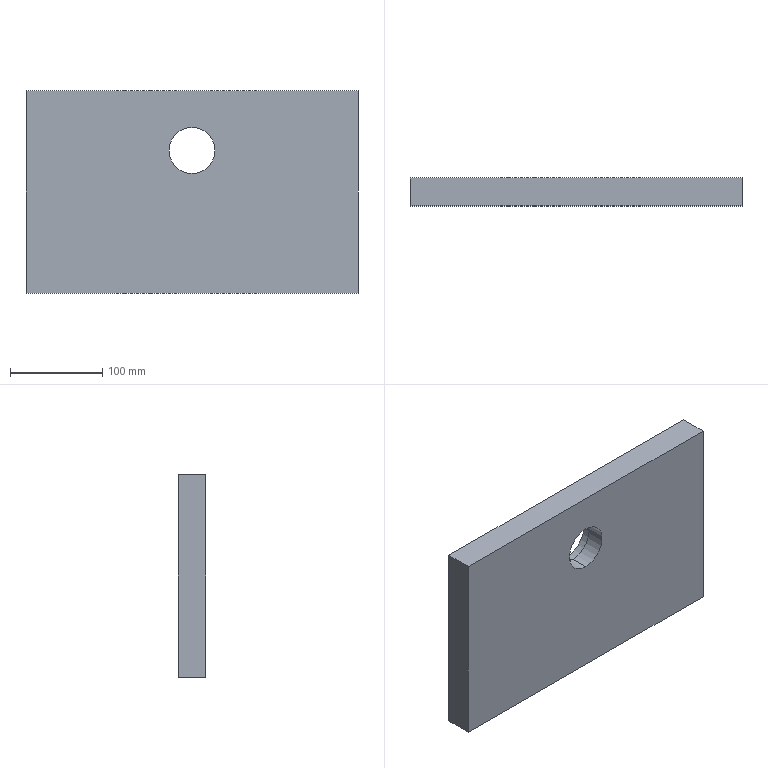Part | SolidWorks | features Cut 2, Extrusion 1 | 1 solid | 11 faces | box 360 x 30 x 220 mm | volume 2312972 mm3 | plane 7 | cylinder 4 | commonest cylinder face diameters 50 x2 55 x2
STEP:
#1=CARTESIAN_POINT('',(0.,0.,20.));
#2=VERTEX_POINT('',#1);
#3=CARTESIAN_POINT('',(0.,0.,70.));
#4=VERTEX_POINT('',#3);
#5=CARTESIAN_POINT('',(0.,0.,45.));
#6=DIRECTION('',(0.,1.,0.));
#7=DIRECTION('',(0.,0.,1.));
#8=AXIS2_PLACEMENT_3D('',#5,#6,#7);
#9=CIRCLE('',#8,25.);
#10=EDGE_CURVE('',#2,#4,#9,.T.);
#11=ORIENTED_EDGE('',*,*,#10,.F.);
#12=CARTESIAN_POINT('',(0.,20.,20.));
#13=VERTEX_POINT('',#12);
#14=CARTESIAN_POINT('',(0.,0.,20.));
#15=DIRECTION('',(0.,1.,0.));
#16=VECTOR('',#15,1000.);
#17=LINE('',#14,#16);
#18=EDGE_CURVE('',#2,#13,#17,.T.);
#19=ORIENTED_EDGE('',*,*,#18,.T.);
#20=CARTESIAN_POINT('',(0.,20.,70.));
#21=VERTEX_POINT('',#20);
#22=CARTESIAN_POINT('',(0.,20.,45.));
#23=DIRECTION('',(0.,1.,0.));
#24=DIRECTION('',(0.,0.,1.));
#25=AXIS2_PLACEMENT_3D('',#22,#23,#24);
#26=CIRCLE('',#25,25.);
#27=EDGE_CURVE('',#13,#21,#26,.T.);
#28=ORIENTED_EDGE('',*,*,#27,.T.);
#29=CARTESIAN_POINT('',(0.,0.,70.));
#30=DIRECTION('',(0.,1.,0.));
#31=VECTOR('',#30,1000.);
#32=LINE('',#29,#31);
#33=EDGE_CURVE('',#4,#21,#32,.T.);
#34=ORIENTED_EDGE('',*,*,#33,.F.);
#35=EDGE_LOOP('',(#11,#19,#28,#34));
#36=FACE_OUTER_BOUND('',#35,.T.);
#37=CARTESIAN_POINT('',(0.,0.,45.));
#38=DIRECTION('',(0.,1.,0.));
#39=DIRECTION('',(0.,0.,1.));
#40=AXIS2_PLACEMENT_3D('',#37,#38,#39);
#41=CYLINDRICAL_SURFACE('',#40,25.);
#42=ADVANCED_FACE('',(#36),#41,.F.);
#43=CARTESIAN_POINT('',(0.,20.,17.5));
#44=VERTEX_POINT('',#43);
#45=CARTESIAN_POINT('',(0.,20.,72.5));
#46=VERTEX_POINT('',#45);
#47=CARTESIAN_POINT('',(0.,20.,45.));
#48=DIRECTION('',(0.,1.,0.));
#49=DIRECTION('',(0.,0.,1.));
#50=AXIS2_PLACEMENT_3D('',#47,#48,#49);
#51=CIRCLE('',#50,27.5);
#52=EDGE_CURVE('',#44,#46,#51,.T.);
#53=ORIENTED_EDGE('',*,*,#52,.F.);
#54=CARTESIAN_POINT('',(0.,30.,17.5));
#55=VERTEX_POINT('',#54);
#56=CARTESIAN_POINT('',(0.,20.,17.5));
#57=DIRECTION('',(0.,1.,0.));
#58=VECTOR('',#57,1000.);
#59=LINE('',#56,#58);
#60=EDGE_CURVE('',#44,#55,#59,.T.);
#61=ORIENTED_EDGE('',*,*,#60,.T.);
#62=CARTESIAN_POINT('',(0.,30.,72.5));
#63=VERTEX_POINT('',#62);
#64=CARTESIAN_POINT('',(0.,30.,45.));
#65=DIRECTION('',(0.,1.,0.));
#66=DIRECTION('',(0.,0.,1.));
#67=AXIS2_PLACEMENT_3D('',#64,#65,#66);
#68=CIRCLE('',#67,27.5);
#69=EDGE_CURVE('',#55,#63,#68,.T.);
#70=ORIENTED_EDGE('',*,*,#69,.T.);
#71=CARTESIAN_POINT('',(0.,20.,72.5));
#72=DIRECTION('',(0.,1.,0.));
#73=VECTOR('',#72,1000.);
#74=LINE('',#71,#73);
#75=EDGE_CURVE('',#46,#63,#74,.T.);
#76=ORIENTED_EDGE('',*,*,#75,.F.);
#77=EDGE_LOOP('',(#53,#61,#70,#76));
#78=FACE_OUTER_BOUND('',#77,.T.);
#79=CARTESIAN_POINT('',(0.,20.,45.));
#80=DIRECTION('',(0.,1.,0.));
#81=DIRECTION('',(0.,0.,1.));
#82=AXIS2_PLACEMENT_3D('',#79,#80,#81);
#83=CYLINDRICAL_SURFACE('',#82,27.5);
#84=ADVANCED_FACE('',(#78),#83,.F.);
#85=CARTESIAN_POINT('',(180.,0.,110.));
#86=VERTEX_POINT('',#85);
#87=CARTESIAN_POINT('',(180.,0.,-110.));
#88=VERTEX_POINT('',#87);
#89=CARTESIAN_POINT('',(180.,0.,110.));
#90=DIRECTION('',(0.,0.,-1.));
#91=VECTOR('',#90,1000.);
#92=LINE('',#89,#91);
#93=EDGE_CURVE('',#86,#88,#92,.T.);
#94=ORIENTED_EDGE('',*,*,#93,.T.);
#95=CARTESIAN_POINT('',(180.,30.,-110.));
#96=VERTEX_POINT('',#95);
#97=CARTESIAN_POINT('',(180.,30.,-110.));
#98=DIRECTION('',(0.,-1.,0.));
#99=VECTOR('',#98,1000.);
#100=LINE('',#97,#99);
#101=EDGE_CURVE('',#96,#88,#100,.T.);
#102=ORIENTED_EDGE('',*,*,#101,.F.);
#103=CARTESIAN_POINT('',(180.,30.,110.));
#104=VERTEX_POINT('',#103);
#105=CARTESIAN_POINT('',(180.,30.,110.));
#106=DIRECTION('',(0.,0.,-1.));
#107=VECTOR('',#106,1000.);
#108=LINE('',#105,#107);
#109=EDGE_CURVE('',#104,#96,#108,.T.);
#110=ORIENTED_EDGE('',*,*,#109,.F.);
#111=CARTESIAN_POINT('',(180.,30.,110.));
#112=DIRECTION('',(0.,-1.,0.));
#113=VECTOR('',#112,1000.);
#114=LINE('',#111,#113);
#115=EDGE_CURVE('',#104,#86,#114,.T.);
#116=ORIENTED_EDGE('',*,*,#115,.T.);
#117=EDGE_LOOP('',(#94,#102,#110,#116));
#118=FACE_OUTER_BOUND('',#117,.T.);
#119=CARTESIAN_POINT('',(180.,30.,110.));
#120=DIRECTION('',(-1.,0.,0.));
#121=DIRECTION('',(0.,0.,1.));
#122=AXIS2_PLACEMENT_3D('',#119,#120,#121);
#123=PLANE('',#122);
#124=ADVANCED_FACE('',(#118),#123,.F.);
#125=CARTESIAN_POINT('',(-180.,0.,-110.));
#126=VERTEX_POINT('',#125);
#127=CARTESIAN_POINT('',(-180.,0.,-110.));
#128=DIRECTION('',(-1.,0.,0.));
#129=VECTOR('',#128,1000.);
#130=LINE('',#127,#129);
#131=EDGE_CURVE('',#88,#126,#130,.T.);
#132=ORIENTED_EDGE('',*,*,#131,.T.);
#133=CARTESIAN_POINT('',(-180.,30.,-110.));
#134=VERTEX_POINT('',#133);
#135=CARTESIAN_POINT('',(-180.,30.,-110.));
#136=DIRECTION('',(0.,-1.,0.));
#137=VECTOR('',#136,1000.);
#138=LINE('',#135,#137);
#139=EDGE_CURVE('',#134,#126,#138,.T.);
#140=ORIENTED_EDGE('',*,*,#139,.F.);
#141=CARTESIAN_POINT('',(-180.,30.,-110.));
#142=DIRECTION('',(-1.,0.,0.));
#143=VECTOR('',#142,1000.);
#144=LINE('',#141,#143);
#145=EDGE_CURVE('',#96,#134,#144,.T.);
#146=ORIENTED_EDGE('',*,*,#145,.F.);
#147=ORIENTED_EDGE('',*,*,#101,.T.);
#148=EDGE_LOOP('',(#132,#140,#146,#147));
#149=FACE_OUTER_BOUND('',#148,.T.);
#150=CARTESIAN_POINT('',(-180.,30.,-110.));
#151=DIRECTION('',(0.,0.,1.));
#152=DIRECTION('',(1.,0.,0.));
#153=AXIS2_PLACEMENT_3D('',#150,#151,#152);
#154=PLANE('',#153);
#155=ADVANCED_FACE('',(#149),#154,.F.);
#156=CARTESIAN_POINT('',(-180.,0.,110.));
#157=VERTEX_POINT('',#156);
#158=CARTESIAN_POINT('',(-180.,0.,110.));
#159=DIRECTION('',(0.,0.,1.));
#160=VECTOR('',#159,1000.);
#161=LINE('',#158,#160);
#162=EDGE_CURVE('',#126,#157,#161,.T.);
#163=ORIENTED_EDGE('',*,*,#162,.T.);
#164=CARTESIAN_POINT('',(-180.,30.,110.));
#165=VERTEX_POINT('',#164);
#166=CARTESIAN_POINT('',(-180.,30.,110.));
#167=DIRECTION('',(0.,-1.,0.));
#168=VECTOR('',#167,1000.);
#169=LINE('',#166,#168);
#170=EDGE_CURVE('',#165,#157,#169,.T.);
#171=ORIENTED_EDGE('',*,*,#170,.F.);
#172=CARTESIAN_POINT('',(-180.,30.,110.));
#173=DIRECTION('',(0.,0.,1.));
#174=VECTOR('',#173,1000.);
#175=LINE('',#172,#174);
#176=EDGE_CURVE('',#134,#165,#175,.T.);
#177=ORIENTED_EDGE('',*,*,#176,.F.);
#178=ORIENTED_EDGE('',*,*,#139,.T.);
#179=EDGE_LOOP('',(#163,#171,#177,#178));
#180=FACE_OUTER_BOUND('',#179,.T.);
#181=CARTESIAN_POINT('',(-180.,30.,110.));
#182=DIRECTION('',(1.,0.,0.));
#183=DIRECTION('',(0.,0.,-1.));
#184=AXIS2_PLACEMENT_3D('',#181,#182,#183);
#185=PLANE('',#184);
#186=ADVANCED_FACE('',(#180),#185,.F.);
#187=CARTESIAN_POINT('',(-180.,0.,110.));
#188=DIRECTION('',(1.,0.,0.));
#189=VECTOR('',#188,1000.);
#190=LINE('',#187,#189);
#191=EDGE_CURVE('',#157,#86,#190,.T.);
#192=ORIENTED_EDGE('',*,*,#191,.T.);
#193=ORIENTED_EDGE('',*,*,#115,.F.);
#194=CARTESIAN_POINT('',(-180.,30.,110.));
#195=DIRECTION('',(1.,0.,0.));
#196=VECTOR('',#195,1000.);
#197=LINE('',#194,#196);
#198=EDGE_CURVE('',#165,#104,#197,.T.);
#199=ORIENTED_EDGE('',*,*,#198,.F.);
#200=ORIENTED_EDGE('',*,*,#170,.T.);
#201=EDGE_LOOP('',(#192,#193,#199,#200));
#202=FACE_OUTER_BOUND('',#201,.T.);
#203=CARTESIAN_POINT('',(-180.,30.,110.));
#204=DIRECTION('',(0.,0.,-1.));
#205=DIRECTION('',(-1.,0.,0.));
#206=AXIS2_PLACEMENT_3D('',#203,#204,#205);
#207=PLANE('',#206);
#208=ADVANCED_FACE('',(#202),#207,.F.);
#209=CARTESIAN_POINT('',(0.,30.,45.));
#210=DIRECTION('',(0.,1.,0.));
#211=DIRECTION('',(0.,0.,1.));
#212=AXIS2_PLACEMENT_3D('',#209,#210,#211);
#213=CIRCLE('',#212,27.5);
#214=EDGE_CURVE('',#63,#55,#213,.T.);
#215=ORIENTED_EDGE('',*,*,#214,.F.);
#216=ORIENTED_EDGE('',*,*,#69,.F.);
#217=EDGE_LOOP('',(#215,#216));
#218=FACE_BOUND('',#217,.T.);
#219=ORIENTED_EDGE('',*,*,#109,.T.);
#220=ORIENTED_EDGE('',*,*,#145,.T.);
#221=ORIENTED_EDGE('',*,*,#176,.T.);
#222=ORIENTED_EDGE('',*,*,#198,.T.);
#223=EDGE_LOOP('',(#219,#220,#221,#222));
#224=FACE_OUTER_BOUND('',#223,.T.);
#225=CARTESIAN_POINT('',(0.,30.,0.));
#226=DIRECTION('',(0.,-1.,0.));
#227=DIRECTION('',(0.,0.,-1.));
#228=AXIS2_PLACEMENT_3D('',#225,#226,#227);
#229=PLANE('',#228);
#230=ADVANCED_FACE('',(#218,#224),#229,.F.);
#231=CARTESIAN_POINT('',(0.,0.,45.));
#232=DIRECTION('',(0.,1.,0.));
#233=DIRECTION('',(0.,0.,1.));
#234=AXIS2_PLACEMENT_3D('',#231,#232,#233);
#235=CIRCLE('',#234,25.);
#236=EDGE_CURVE('',#4,#2,#235,.T.);
#237=ORIENTED_EDGE('',*,*,#236,.T.);
#238=ORIENTED_EDGE('',*,*,#10,.T.);
#239=EDGE_LOOP('',(#237,#238));
#240=FACE_BOUND('',#239,.T.);
#241=ORIENTED_EDGE('',*,*,#93,.F.);
#242=ORIENTED_EDGE('',*,*,#191,.F.);
#243=ORIENTED_EDGE('',*,*,#162,.F.);
#244=ORIENTED_EDGE('',*,*,#131,.F.);
#245=EDGE_LOOP('',(#241,#242,#243,#244));
#246=FACE_OUTER_BOUND('',#245,.T.);
#247=CARTESIAN_POINT('',(0.,0.,0.));
#248=DIRECTION('',(0.,-1.,0.));
#249=DIRECTION('',(0.,0.,-1.));
#250=AXIS2_PLACEMENT_3D('',#247,#248,#249);
#251=PLANE('',#250);
#252=ADVANCED_FACE('',(#240,#246),#251,.T.);
#253=ORIENTED_EDGE('',*,*,#60,.F.);
#254=CARTESIAN_POINT('',(0.,20.,45.));
#255=DIRECTION('',(0.,1.,0.));
#256=DIRECTION('',(0.,0.,1.));
#257=AXIS2_PLACEMENT_3D('',#254,#255,#256);
#258=CIRCLE('',#257,27.5);
#259=EDGE_CURVE('',#46,#44,#258,.T.);
#260=ORIENTED_EDGE('',*,*,#259,.F.);
#261=ORIENTED_EDGE('',*,*,#75,.T.);
#262=ORIENTED_EDGE('',*,*,#214,.T.);
#263=EDGE_LOOP('',(#253,#260,#261,#262));
#264=FACE_OUTER_BOUND('',#263,.T.);
#265=CARTESIAN_POINT('',(0.,20.,45.));
#266=DIRECTION('',(0.,1.,0.));
#267=DIRECTION('',(0.,0.,1.));
#268=AXIS2_PLACEMENT_3D('',#265,#266,#267);
#269=CYLINDRICAL_SURFACE('',#268,27.5);
#270=ADVANCED_FACE('',(#264),#269,.F.);
#271=CARTESIAN_POINT('',(0.,20.,45.));
#272=DIRECTION('',(0.,1.,0.));
#273=DIRECTION('',(0.,0.,1.));
#274=AXIS2_PLACEMENT_3D('',#271,#272,#273);
#275=CIRCLE('',#274,25.);
#276=EDGE_CURVE('',#21,#13,#275,.T.);
#277=ORIENTED_EDGE('',*,*,#276,.F.);
#278=ORIENTED_EDGE('',*,*,#27,.F.);
#279=EDGE_LOOP('',(#277,#278));
#280=FACE_BOUND('',#279,.T.);
#281=ORIENTED_EDGE('',*,*,#259,.T.);
#282=ORIENTED_EDGE('',*,*,#52,.T.);
#283=EDGE_LOOP('',(#281,#282));
#284=FACE_OUTER_BOUND('',#283,.T.);
#285=CARTESIAN_POINT('',(0.,20.,45.));
#286=DIRECTION('',(0.,1.,0.));
#287=DIRECTION('',(0.,0.,1.));
#288=AXIS2_PLACEMENT_3D('',#285,#286,#287);
#289=PLANE('',#288);
#290=ADVANCED_FACE('',(#280,#284),#289,.T.);
#291=ORIENTED_EDGE('',*,*,#18,.F.);
#292=ORIENTED_EDGE('',*,*,#236,.F.);
#293=ORIENTED_EDGE('',*,*,#33,.T.);
#294=ORIENTED_EDGE('',*,*,#276,.T.);
#295=EDGE_LOOP('',(#291,#292,#293,#294));
#296=FACE_OUTER_BOUND('',#295,.T.);
#297=CARTESIAN_POINT('',(0.,0.,45.));
#298=DIRECTION('',(0.,1.,0.));
#299=DIRECTION('',(0.,0.,1.));
#300=AXIS2_PLACEMENT_3D('',#297,#298,#299);
#301=CYLINDRICAL_SURFACE('',#300,25.);
#302=ADVANCED_FACE('',(#296),#301,.F.);
#303=CLOSED_SHELL('',(#42,#84,#124,#155,#186,#208,#230,#252,#270,#290,#302));
#304=MANIFOLD_SOLID_BREP('',#303);
#305=CARTESIAN_POINT('',(0.,0.,0.));
#306=DIRECTION('',(0.,0.,1.));
#307=DIRECTION('',(1.,0.,0.));
#308=AXIS2_PLACEMENT_3D('',#305,#306,#307);
#309=(LENGTH_UNIT()NAMED_UNIT(*)SI_UNIT(.MILLI.,.METRE.));
#310=UNCERTAINTY_MEASURE_WITH_UNIT(LENGTH_MEASURE(0.00001),#309,'','');
#311=(NAMED_UNIT(*)PLANE_ANGLE_UNIT()SI_UNIT($,.RADIAN.));
#312=(NAMED_UNIT(*)SI_UNIT($,.STERADIAN.)SOLID_ANGLE_UNIT());
#313=(GEOMETRIC_REPRESENTATION_CONTEXT(3)GLOBAL_UNCERTAINTY_ASSIGNED_CONTEXT((#310))GLOBAL_UNIT_ASSIGNED_CONTEXT((#309,#311,#312))REPRESENTATION_CONTEXT('',''));
#314=ADVANCED_BREP_SHAPE_REPRESENTATION('',(#304,#308),#313);